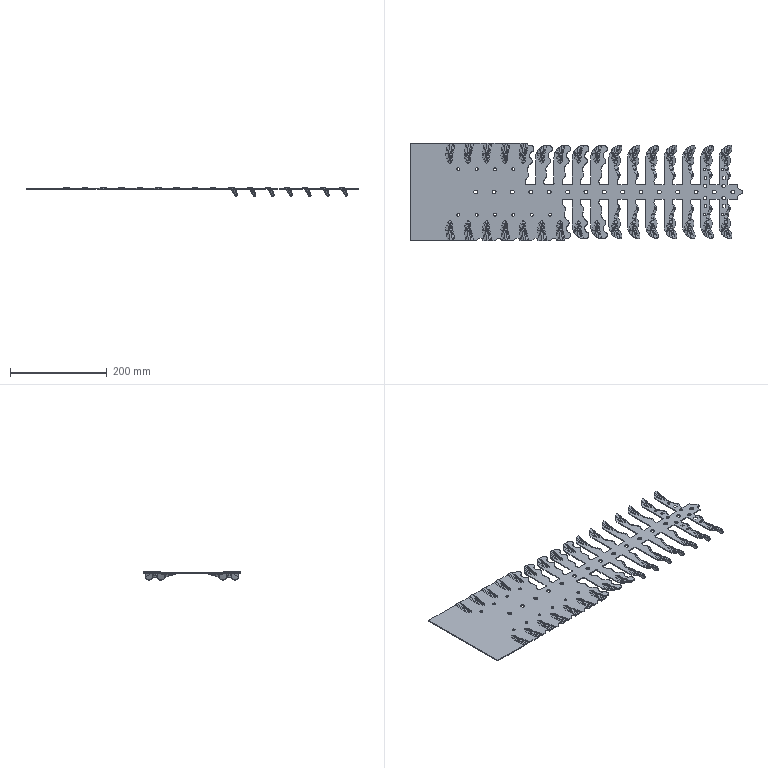Part | STEP file | 1 solid | 4033 faces | volume 214873 mm3 | spline 2524 | plane 1252 | cylinder 161 | sphere 64 | torus 18 | other 14 | commonest cylinder face diameters 6 x41 12 x22 1 x16 8.1 x15 10 x14 13.815 x14